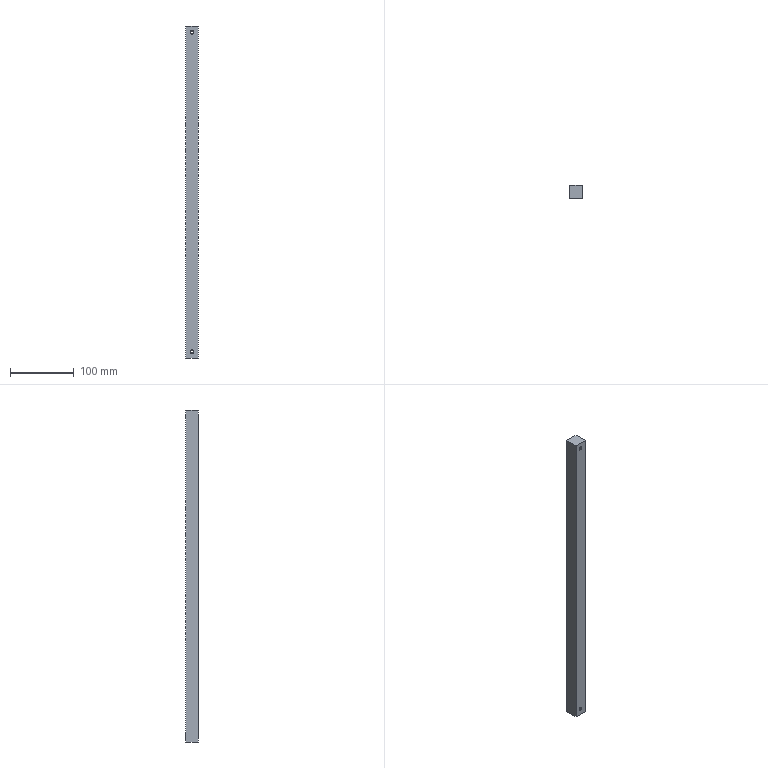Part | STEP file | Inner slide strip | 1 solid | 18 faces | box 20 x 20 x 520 mm | volume 207468 mm3 | cone 8 | plane 6 | cylinder 4 | commonest cylinder face diameters 4 x4
STEP:
#1=CARTESIAN_POINT('',(-3.247,0.9353,508.));
#2=VERTEX_POINT('',#1);
#3=CARTESIAN_POINT('',(-5.247,0.9353,510.));
#4=VERTEX_POINT('',#3);
#5=CARTESIAN_POINT('',(-3.247,0.9353,510.));
#6=DIRECTION('',(0.,1.,0.));
#7=DIRECTION('',(0.,0.,1.));
#8=AXIS2_PLACEMENT_3D('',#5,#6,#7);
#9=CIRCLE('',#8,2.);
#10=EDGE_CURVE('',#2,#4,#9,.T.);
#11=ORIENTED_EDGE('',*,*,#10,.F.);
#12=CARTESIAN_POINT('',(-3.247,1.935,507.));
#13=VERTEX_POINT('',#12);
#14=CARTESIAN_POINT('',(-3.247,1.935,507.));
#15=DIRECTION('',(0.,0.7071,-0.7071));
#16=VECTOR('',#15,1000.);
#17=LINE('',#14,#16);
#18=EDGE_CURVE('',#2,#13,#17,.T.);
#19=ORIENTED_EDGE('',*,*,#18,.T.);
#20=CARTESIAN_POINT('',(-3.247,1.935,513.));
#21=VERTEX_POINT('',#20);
#22=CARTESIAN_POINT('',(-3.247,1.935,510.));
#23=DIRECTION('',(0.,1.,0.));
#24=DIRECTION('',(0.,0.,1.));
#25=AXIS2_PLACEMENT_3D('',#22,#23,#24);
#26=CIRCLE('',#25,3.);
#27=EDGE_CURVE('',#13,#21,#26,.T.);
#28=ORIENTED_EDGE('',*,*,#27,.T.);
#29=CARTESIAN_POINT('',(-3.247,0.9353,512.));
#30=VERTEX_POINT('',#29);
#31=CARTESIAN_POINT('',(-3.247,1.935,513.));
#32=DIRECTION('',(0.,0.7071,0.7071));
#33=VECTOR('',#32,1000.);
#34=LINE('',#31,#33);
#35=EDGE_CURVE('',#30,#21,#34,.T.);
#36=ORIENTED_EDGE('',*,*,#35,.F.);
#37=CARTESIAN_POINT('',(-3.247,0.9353,510.));
#38=DIRECTION('',(0.,1.,0.));
#39=DIRECTION('',(0.,0.,1.));
#40=AXIS2_PLACEMENT_3D('',#37,#38,#39);
#41=CIRCLE('',#40,2.);
#42=EDGE_CURVE('',#4,#30,#41,.T.);
#43=ORIENTED_EDGE('',*,*,#42,.F.);
#44=EDGE_LOOP('',(#11,#19,#28,#36,#43));
#45=FACE_OUTER_BOUND('',#44,.T.);
#46=CARTESIAN_POINT('',(-3.247,1.935,510.));
#47=DIRECTION('',(0.,1.,0.));
#48=DIRECTION('',(0.,0.,1.));
#49=AXIS2_PLACEMENT_3D('',#46,#47,#48);
#50=CONICAL_SURFACE('',#49,3.,0.7854);
#51=ADVANCED_FACE('',(#45),#50,.F.);
#52=CARTESIAN_POINT('',(-3.247,0.9353,8.));
#53=VERTEX_POINT('',#52);
#54=CARTESIAN_POINT('',(-5.247,0.9353,10.));
#55=VERTEX_POINT('',#54);
#56=CARTESIAN_POINT('',(-3.247,0.9353,10.));
#57=DIRECTION('',(0.,1.,0.));
#58=DIRECTION('',(0.,0.,1.));
#59=AXIS2_PLACEMENT_3D('',#56,#57,#58);
#60=CIRCLE('',#59,2.);
#61=EDGE_CURVE('',#53,#55,#60,.T.);
#62=ORIENTED_EDGE('',*,*,#61,.F.);
#63=CARTESIAN_POINT('',(-3.247,1.935,7.));
#64=VERTEX_POINT('',#63);
#65=CARTESIAN_POINT('',(-3.247,1.935,7.));
#66=DIRECTION('',(0.,0.7071,-0.7071));
#67=VECTOR('',#66,1000.);
#68=LINE('',#65,#67);
#69=EDGE_CURVE('',#53,#64,#68,.T.);
#70=ORIENTED_EDGE('',*,*,#69,.T.);
#71=CARTESIAN_POINT('',(-3.247,1.935,13.));
#72=VERTEX_POINT('',#71);
#73=CARTESIAN_POINT('',(-3.247,1.935,10.));
#74=DIRECTION('',(0.,1.,0.));
#75=DIRECTION('',(0.,0.,1.));
#76=AXIS2_PLACEMENT_3D('',#73,#74,#75);
#77=CIRCLE('',#76,3.);
#78=EDGE_CURVE('',#64,#72,#77,.T.);
#79=ORIENTED_EDGE('',*,*,#78,.T.);
#80=CARTESIAN_POINT('',(-3.247,0.9353,12.));
#81=VERTEX_POINT('',#80);
#82=CARTESIAN_POINT('',(-3.247,1.935,13.));
#83=DIRECTION('',(0.,0.7071,0.7071));
#84=VECTOR('',#83,1000.);
#85=LINE('',#82,#84);
#86=EDGE_CURVE('',#81,#72,#85,.T.);
#87=ORIENTED_EDGE('',*,*,#86,.F.);
#88=CARTESIAN_POINT('',(-3.247,0.9353,10.));
#89=DIRECTION('',(0.,1.,0.));
#90=DIRECTION('',(0.,0.,1.));
#91=AXIS2_PLACEMENT_3D('',#88,#89,#90);
#92=CIRCLE('',#91,2.);
#93=EDGE_CURVE('',#55,#81,#92,.T.);
#94=ORIENTED_EDGE('',*,*,#93,.F.);
#95=EDGE_LOOP('',(#62,#70,#79,#87,#94));
#96=FACE_OUTER_BOUND('',#95,.T.);
#97=CARTESIAN_POINT('',(-3.247,1.935,10.));
#98=DIRECTION('',(0.,1.,0.));
#99=DIRECTION('',(0.,0.,1.));
#100=AXIS2_PLACEMENT_3D('',#97,#98,#99);
#101=CONICAL_SURFACE('',#100,3.,0.7854);
#102=ADVANCED_FACE('',(#96),#101,.F.);
#103=CARTESIAN_POINT('',(-3.247,-17.065,12.));
#104=VERTEX_POINT('',#103);
#105=CARTESIAN_POINT('',(-5.247,-17.065,10.));
#106=VERTEX_POINT('',#105);
#107=CARTESIAN_POINT('',(-3.247,-17.065,10.));
#108=DIRECTION('',(0.,-1.,0.));
#109=DIRECTION('',(0.,0.,-1.));
#110=AXIS2_PLACEMENT_3D('',#107,#108,#109);
#111=CIRCLE('',#110,2.);
#112=EDGE_CURVE('',#104,#106,#111,.T.);
#113=ORIENTED_EDGE('',*,*,#112,.F.);
#114=CARTESIAN_POINT('',(-3.247,-18.065,13.));
#115=VERTEX_POINT('',#114);
#116=CARTESIAN_POINT('',(-3.247,-18.065,13.));
#117=DIRECTION('',(0.,-0.7071,0.7071));
#118=VECTOR('',#117,1000.);
#119=LINE('',#116,#118);
#120=EDGE_CURVE('',#104,#115,#119,.T.);
#121=ORIENTED_EDGE('',*,*,#120,.T.);
#122=CARTESIAN_POINT('',(-3.247,-18.065,7.));
#123=VERTEX_POINT('',#122);
#124=CARTESIAN_POINT('',(-3.247,-18.065,10.));
#125=DIRECTION('',(0.,-1.,0.));
#126=DIRECTION('',(0.,0.,-1.));
#127=AXIS2_PLACEMENT_3D('',#124,#125,#126);
#128=CIRCLE('',#127,3.);
#129=EDGE_CURVE('',#115,#123,#128,.T.);
#130=ORIENTED_EDGE('',*,*,#129,.T.);
#131=CARTESIAN_POINT('',(-3.247,-17.065,8.));
#132=VERTEX_POINT('',#131);
#133=CARTESIAN_POINT('',(-3.247,-18.065,7.));
#134=DIRECTION('',(0.,-0.7071,-0.7071));
#135=VECTOR('',#134,1000.);
#136=LINE('',#133,#135);
#137=EDGE_CURVE('',#132,#123,#136,.T.);
#138=ORIENTED_EDGE('',*,*,#137,.F.);
#139=CARTESIAN_POINT('',(-3.247,-17.065,10.));
#140=DIRECTION('',(0.,-1.,0.));
#141=DIRECTION('',(0.,0.,-1.));
#142=AXIS2_PLACEMENT_3D('',#139,#140,#141);
#143=CIRCLE('',#142,2.);
#144=EDGE_CURVE('',#106,#132,#143,.T.);
#145=ORIENTED_EDGE('',*,*,#144,.F.);
#146=EDGE_LOOP('',(#113,#121,#130,#138,#145));
#147=FACE_OUTER_BOUND('',#146,.T.);
#148=CARTESIAN_POINT('',(-3.247,-18.065,10.));
#149=DIRECTION('',(0.,-1.,0.));
#150=DIRECTION('',(0.,0.,-1.));
#151=AXIS2_PLACEMENT_3D('',#148,#149,#150);
#152=CONICAL_SURFACE('',#151,3.,0.7854);
#153=ADVANCED_FACE('',(#147),#152,.F.);
#154=CARTESIAN_POINT('',(-3.247,-17.065,512.));
#155=VERTEX_POINT('',#154);
#156=CARTESIAN_POINT('',(-5.247,-17.065,510.));
#157=VERTEX_POINT('',#156);
#158=CARTESIAN_POINT('',(-3.247,-17.065,510.));
#159=DIRECTION('',(0.,-1.,0.));
#160=DIRECTION('',(0.,0.,-1.));
#161=AXIS2_PLACEMENT_3D('',#158,#159,#160);
#162=CIRCLE('',#161,2.);
#163=EDGE_CURVE('',#155,#157,#162,.T.);
#164=ORIENTED_EDGE('',*,*,#163,.F.);
#165=CARTESIAN_POINT('',(-3.247,-18.065,513.));
#166=VERTEX_POINT('',#165);
#167=CARTESIAN_POINT('',(-3.247,-18.065,513.));
#168=DIRECTION('',(0.,-0.7071,0.7071));
#169=VECTOR('',#168,1000.);
#170=LINE('',#167,#169);
#171=EDGE_CURVE('',#155,#166,#170,.T.);
#172=ORIENTED_EDGE('',*,*,#171,.T.);
#173=CARTESIAN_POINT('',(-3.247,-18.065,507.));
#174=VERTEX_POINT('',#173);
#175=CARTESIAN_POINT('',(-3.247,-18.065,510.));
#176=DIRECTION('',(0.,-1.,0.));
#177=DIRECTION('',(0.,0.,-1.));
#178=AXIS2_PLACEMENT_3D('',#175,#176,#177);
#179=CIRCLE('',#178,3.);
#180=EDGE_CURVE('',#166,#174,#179,.T.);
#181=ORIENTED_EDGE('',*,*,#180,.T.);
#182=CARTESIAN_POINT('',(-3.247,-17.065,508.));
#183=VERTEX_POINT('',#182);
#184=CARTESIAN_POINT('',(-3.247,-18.065,507.));
#185=DIRECTION('',(0.,-0.7071,-0.7071));
#186=VECTOR('',#185,1000.);
#187=LINE('',#184,#186);
#188=EDGE_CURVE('',#183,#174,#187,.T.);
#189=ORIENTED_EDGE('',*,*,#188,.F.);
#190=CARTESIAN_POINT('',(-3.247,-17.065,510.));
#191=DIRECTION('',(0.,-1.,0.));
#192=DIRECTION('',(0.,0.,-1.));
#193=AXIS2_PLACEMENT_3D('',#190,#191,#192);
#194=CIRCLE('',#193,2.);
#195=EDGE_CURVE('',#157,#183,#194,.T.);
#196=ORIENTED_EDGE('',*,*,#195,.F.);
#197=EDGE_LOOP('',(#164,#172,#181,#189,#196));
#198=FACE_OUTER_BOUND('',#197,.T.);
#199=CARTESIAN_POINT('',(-3.247,-18.065,510.));
#200=DIRECTION('',(0.,-1.,0.));
#201=DIRECTION('',(0.,0.,-1.));
#202=AXIS2_PLACEMENT_3D('',#199,#200,#201);
#203=CONICAL_SURFACE('',#202,3.,0.7854);
#204=ADVANCED_FACE('',(#198),#203,.F.);
#205=ORIENTED_EDGE('',*,*,#195,.T.);
#206=CARTESIAN_POINT('',(-1.247,-17.065,510.));
#207=VERTEX_POINT('',#206);
#208=CARTESIAN_POINT('',(-3.247,-17.065,510.));
#209=DIRECTION('',(0.,-1.,0.));
#210=DIRECTION('',(0.,0.,-1.));
#211=AXIS2_PLACEMENT_3D('',#208,#209,#210);
#212=CIRCLE('',#211,2.);
#213=EDGE_CURVE('',#183,#207,#212,.T.);
#214=ORIENTED_EDGE('',*,*,#213,.T.);
#215=CARTESIAN_POINT('',(-1.247,0.9353,510.));
#216=VERTEX_POINT('',#215);
#217=CARTESIAN_POINT('',(-1.247,-18.065,510.));
#218=DIRECTION('',(0.,1.,0.));
#219=VECTOR('',#218,1000.);
#220=LINE('',#217,#219);
#221=EDGE_CURVE('',#207,#216,#220,.T.);
#222=ORIENTED_EDGE('',*,*,#221,.T.);
#223=CARTESIAN_POINT('',(-3.247,0.9353,510.));
#224=DIRECTION('',(0.,1.,0.));
#225=DIRECTION('',(0.,0.,1.));
#226=AXIS2_PLACEMENT_3D('',#223,#224,#225);
#227=CIRCLE('',#226,2.);
#228=EDGE_CURVE('',#216,#2,#227,.T.);
#229=ORIENTED_EDGE('',*,*,#228,.T.);
#230=ORIENTED_EDGE('',*,*,#10,.T.);
#231=CARTESIAN_POINT('',(-5.247,-18.065,510.));
#232=DIRECTION('',(0.,1.,0.));
#233=VECTOR('',#232,1000.);
#234=LINE('',#231,#233);
#235=EDGE_CURVE('',#157,#4,#234,.T.);
#236=ORIENTED_EDGE('',*,*,#235,.F.);
#237=EDGE_LOOP('',(#205,#214,#222,#229,#230,#236));
#238=FACE_OUTER_BOUND('',#237,.T.);
#239=CARTESIAN_POINT('',(-3.247,-18.065,510.));
#240=DIRECTION('',(0.,1.,0.));
#241=DIRECTION('',(-1.,0.,0.));
#242=AXIS2_PLACEMENT_3D('',#239,#240,#241);
#243=CYLINDRICAL_SURFACE('',#242,2.);
#244=ADVANCED_FACE('',(#238),#243,.F.);
#245=ORIENTED_EDGE('',*,*,#144,.T.);
#246=CARTESIAN_POINT('',(-1.247,-17.065,10.));
#247=VERTEX_POINT('',#246);
#248=CARTESIAN_POINT('',(-3.247,-17.065,10.));
#249=DIRECTION('',(0.,-1.,0.));
#250=DIRECTION('',(0.,0.,-1.));
#251=AXIS2_PLACEMENT_3D('',#248,#249,#250);
#252=CIRCLE('',#251,2.);
#253=EDGE_CURVE('',#132,#247,#252,.T.);
#254=ORIENTED_EDGE('',*,*,#253,.T.);
#255=CARTESIAN_POINT('',(-1.247,0.9353,10.));
#256=VERTEX_POINT('',#255);
#257=CARTESIAN_POINT('',(-1.247,-18.065,10.));
#258=DIRECTION('',(0.,1.,0.));
#259=VECTOR('',#258,1000.);
#260=LINE('',#257,#259);
#261=EDGE_CURVE('',#247,#256,#260,.T.);
#262=ORIENTED_EDGE('',*,*,#261,.T.);
#263=CARTESIAN_POINT('',(-3.247,0.9353,10.));
#264=DIRECTION('',(0.,1.,0.));
#265=DIRECTION('',(0.,0.,1.));
#266=AXIS2_PLACEMENT_3D('',#263,#264,#265);
#267=CIRCLE('',#266,2.);
#268=EDGE_CURVE('',#256,#53,#267,.T.);
#269=ORIENTED_EDGE('',*,*,#268,.T.);
#270=ORIENTED_EDGE('',*,*,#61,.T.);
#271=CARTESIAN_POINT('',(-5.247,-18.065,10.));
#272=DIRECTION('',(0.,1.,0.));
#273=VECTOR('',#272,1000.);
#274=LINE('',#271,#273);
#275=EDGE_CURVE('',#106,#55,#274,.T.);
#276=ORIENTED_EDGE('',*,*,#275,.F.);
#277=EDGE_LOOP('',(#245,#254,#262,#269,#270,#276));
#278=FACE_OUTER_BOUND('',#277,.T.);
#279=CARTESIAN_POINT('',(-3.247,-18.065,10.));
#280=DIRECTION('',(0.,1.,0.));
#281=DIRECTION('',(-1.,0.,0.));
#282=AXIS2_PLACEMENT_3D('',#279,#280,#281);
#283=CYLINDRICAL_SURFACE('',#282,2.);
#284=ADVANCED_FACE('',(#278),#283,.F.);
#285=CARTESIAN_POINT('',(6.753,1.935,520.));
#286=VERTEX_POINT('',#285);
#287=CARTESIAN_POINT('',(6.753,1.935,0.));
#288=VERTEX_POINT('',#287);
#289=CARTESIAN_POINT('',(6.753,1.935,520.));
#290=DIRECTION('',(0.,0.,-1.));
#291=VECTOR('',#290,1000.);
#292=LINE('',#289,#291);
#293=EDGE_CURVE('',#286,#288,#292,.T.);
#294=ORIENTED_EDGE('',*,*,#293,.F.);
#295=CARTESIAN_POINT('',(6.753,-18.065,520.));
#296=VERTEX_POINT('',#295);
#297=CARTESIAN_POINT('',(6.753,1.935,520.));
#298=DIRECTION('',(0.,1.,0.));
#299=VECTOR('',#298,1000.);
#300=LINE('',#297,#299);
#301=EDGE_CURVE('',#296,#286,#300,.T.);
#302=ORIENTED_EDGE('',*,*,#301,.F.);
#303=CARTESIAN_POINT('',(6.753,-18.065,0.));
#304=VERTEX_POINT('',#303);
#305=CARTESIAN_POINT('',(6.753,-18.065,520.));
#306=DIRECTION('',(0.,0.,1.));
#307=VECTOR('',#306,1000.);
#308=LINE('',#305,#307);
#309=EDGE_CURVE('',#304,#296,#308,.T.);
#310=ORIENTED_EDGE('',*,*,#309,.F.);
#311=CARTESIAN_POINT('',(6.753,1.935,0.));
#312=DIRECTION('',(0.,-1.,0.));
#313=VECTOR('',#312,1000.);
#314=LINE('',#311,#313);
#315=EDGE_CURVE('',#288,#304,#314,.T.);
#316=ORIENTED_EDGE('',*,*,#315,.F.);
#317=EDGE_LOOP('',(#294,#302,#310,#316));
#318=FACE_OUTER_BOUND('',#317,.T.);
#319=CARTESIAN_POINT('',(6.753,1.935,520.));
#320=DIRECTION('',(-1.,0.,0.));
#321=DIRECTION('',(0.,0.,1.));
#322=AXIS2_PLACEMENT_3D('',#319,#320,#321);
#323=PLANE('',#322);
#324=ADVANCED_FACE('',(#318),#323,.F.);
#325=CARTESIAN_POINT('',(-13.247,1.935,0.));
#326=VERTEX_POINT('',#325);
#327=CARTESIAN_POINT('',(-13.247,1.935,0.));
#328=DIRECTION('',(-1.,0.,0.));
#329=VECTOR('',#328,1000.);
#330=LINE('',#327,#329);
#331=EDGE_CURVE('',#288,#326,#330,.T.);
#332=ORIENTED_EDGE('',*,*,#331,.F.);
#333=ORIENTED_EDGE('',*,*,#315,.T.);
#334=CARTESIAN_POINT('',(-13.247,-18.065,0.));
#335=VERTEX_POINT('',#334);
#336=CARTESIAN_POINT('',(-13.247,-18.065,0.));
#337=DIRECTION('',(1.,0.,0.));
#338=VECTOR('',#337,1000.);
#339=LINE('',#336,#338);
#340=EDGE_CURVE('',#335,#304,#339,.T.);
#341=ORIENTED_EDGE('',*,*,#340,.F.);
#342=CARTESIAN_POINT('',(-13.247,-18.065,0.));
#343=DIRECTION('',(0.,-1.,0.));
#344=VECTOR('',#343,1000.);
#345=LINE('',#342,#344);
#346=EDGE_CURVE('',#326,#335,#345,.T.);
#347=ORIENTED_EDGE('',*,*,#346,.F.);
#348=EDGE_LOOP('',(#332,#333,#341,#347));
#349=FACE_OUTER_BOUND('',#348,.T.);
#350=CARTESIAN_POINT('',(-13.247,-18.065,0.));
#351=DIRECTION('',(0.,0.,1.));
#352=DIRECTION('',(1.,0.,0.));
#353=AXIS2_PLACEMENT_3D('',#350,#351,#352);
#354=PLANE('',#353);
#355=ADVANCED_FACE('',(#349),#354,.F.);
#356=CARTESIAN_POINT('',(-13.247,1.935,520.));
#357=VERTEX_POINT('',#356);
#358=CARTESIAN_POINT('',(-13.247,1.935,520.));
#359=DIRECTION('',(0.,0.,-1.));
#360=VECTOR('',#359,1000.);
#361=LINE('',#358,#360);
#362=EDGE_CURVE('',#357,#326,#361,.T.);
#363=ORIENTED_EDGE('',*,*,#362,.F.);
#364=CARTESIAN_POINT('',(-13.247,1.935,520.));
#365=DIRECTION('',(-1.,0.,0.));
#366=VECTOR('',#365,1000.);
#367=LINE('',#364,#366);
#368=EDGE_CURVE('',#286,#357,#367,.T.);
#369=ORIENTED_EDGE('',*,*,#368,.F.);
#370=ORIENTED_EDGE('',*,*,#293,.T.);
#371=ORIENTED_EDGE('',*,*,#331,.T.);
#372=EDGE_LOOP('',(#363,#369,#370,#371));
#373=FACE_OUTER_BOUND('',#372,.T.);
#374=CARTESIAN_POINT('',(-3.247,1.935,510.));
#375=DIRECTION('',(0.,1.,0.));
#376=DIRECTION('',(0.,0.,1.));
#377=AXIS2_PLACEMENT_3D('',#374,#375,#376);
#378=CIRCLE('',#377,3.);
#379=EDGE_CURVE('',#21,#13,#378,.T.);
#380=ORIENTED_EDGE('',*,*,#379,.F.);
#381=ORIENTED_EDGE('',*,*,#27,.F.);
#382=EDGE_LOOP('',(#380,#381));
#383=FACE_BOUND('',#382,.T.);
#384=CARTESIAN_POINT('',(-3.247,1.935,10.));
#385=DIRECTION('',(0.,1.,0.));
#386=DIRECTION('',(0.,0.,1.));
#387=AXIS2_PLACEMENT_3D('',#384,#385,#386);
#388=CIRCLE('',#387,3.);
#389=EDGE_CURVE('',#72,#64,#388,.T.);
#390=ORIENTED_EDGE('',*,*,#389,.F.);
#391=ORIENTED_EDGE('',*,*,#78,.F.);
#392=EDGE_LOOP('',(#390,#391));
#393=FACE_BOUND('',#392,.T.);
#394=CARTESIAN_POINT('',(-13.247,1.935,520.));
#395=DIRECTION('',(0.,-1.,0.));
#396=DIRECTION('',(1.,0.,0.));
#397=AXIS2_PLACEMENT_3D('',#394,#395,#396);
#398=PLANE('',#397);
#399=ADVANCED_FACE('',(#373,#383,#393),#398,.F.);
#400=ORIENTED_EDGE('',*,*,#301,.T.);
#401=ORIENTED_EDGE('',*,*,#368,.T.);
#402=CARTESIAN_POINT('',(-13.247,-18.065,520.));
#403=VERTEX_POINT('',#402);
#404=CARTESIAN_POINT('',(-13.247,-18.065,520.));
#405=DIRECTION('',(0.,-1.,0.));
#406=VECTOR('',#405,1000.);
#407=LINE('',#404,#406);
#408=EDGE_CURVE('',#357,#403,#407,.T.);
#409=ORIENTED_EDGE('',*,*,#408,.T.);
#410=CARTESIAN_POINT('',(-13.247,-18.065,520.));
#411=DIRECTION('',(1.,0.,0.));
#412=VECTOR('',#411,1000.);
#413=LINE('',#410,#412);
#414=EDGE_CURVE('',#403,#296,#413,.T.);
#415=ORIENTED_EDGE('',*,*,#414,.T.);
#416=EDGE_LOOP('',(#400,#401,#409,#415));
#417=FACE_OUTER_BOUND('',#416,.T.);
#418=CARTESIAN_POINT('',(-13.247,-18.065,520.));
#419=DIRECTION('',(0.,0.,1.));
#420=DIRECTION('',(1.,0.,0.));
#421=AXIS2_PLACEMENT_3D('',#418,#419,#420);
#422=PLANE('',#421);
#423=ADVANCED_FACE('',(#417),#422,.T.);
#424=ORIENTED_EDGE('',*,*,#309,.T.);
#425=ORIENTED_EDGE('',*,*,#414,.F.);
#426=CARTESIAN_POINT('',(-13.247,-18.065,520.));
#427=DIRECTION('',(0.,0.,1.));
#428=VECTOR('',#427,1000.);
#429=LINE('',#426,#428);
#430=EDGE_CURVE('',#335,#403,#429,.T.);
#431=ORIENTED_EDGE('',*,*,#430,.F.);
#432=ORIENTED_EDGE('',*,*,#340,.T.);
#433=EDGE_LOOP('',(#424,#425,#431,#432));
#434=FACE_OUTER_BOUND('',#433,.T.);
#435=CARTESIAN_POINT('',(-3.247,-18.065,10.));
#436=DIRECTION('',(0.,-1.,0.));
#437=DIRECTION('',(0.,0.,-1.));
#438=AXIS2_PLACEMENT_3D('',#435,#436,#437);
#439=CIRCLE('',#438,3.);
#440=EDGE_CURVE('',#123,#115,#439,.T.);
#441=ORIENTED_EDGE('',*,*,#440,.F.);
#442=ORIENTED_EDGE('',*,*,#129,.F.);
#443=EDGE_LOOP('',(#441,#442));
#444=FACE_BOUND('',#443,.T.);
#445=CARTESIAN_POINT('',(-3.247,-18.065,510.));
#446=DIRECTION('',(0.,-1.,0.));
#447=DIRECTION('',(0.,0.,-1.));
#448=AXIS2_PLACEMENT_3D('',#445,#446,#447);
#449=CIRCLE('',#448,3.);
#450=EDGE_CURVE('',#174,#166,#449,.T.);
#451=ORIENTED_EDGE('',*,*,#450,.F.);
#452=ORIENTED_EDGE('',*,*,#180,.F.);
#453=EDGE_LOOP('',(#451,#452));
#454=FACE_BOUND('',#453,.T.);
#455=CARTESIAN_POINT('',(-13.247,-18.065,520.));
#456=DIRECTION('',(0.,1.,0.));
#457=DIRECTION('',(0.,0.,1.));
#458=AXIS2_PLACEMENT_3D('',#455,#456,#457);
#459=PLANE('',#458);
#460=ADVANCED_FACE('',(#434,#444,#454),#459,.F.);
#461=ORIENTED_EDGE('',*,*,#430,.T.);
#462=ORIENTED_EDGE('',*,*,#408,.F.);
#463=ORIENTED_EDGE('',*,*,#362,.T.);
#464=ORIENTED_EDGE('',*,*,#346,.T.);
#465=EDGE_LOOP('',(#461,#462,#463,#464));
#466=FACE_OUTER_BOUND('',#465,.T.);
#467=CARTESIAN_POINT('',(-13.247,1.935,520.));
#468=DIRECTION('',(1.,0.,0.));
#469=DIRECTION('',(0.,0.,-1.));
#470=AXIS2_PLACEMENT_3D('',#467,#468,#469);
#471=PLANE('',#470);
#472=ADVANCED_FACE('',(#466),#471,.F.);
#473=ORIENTED_EDGE('',*,*,#18,.F.);
#474=ORIENTED_EDGE('',*,*,#228,.F.);
#475=CARTESIAN_POINT('',(-3.247,0.9353,510.));
#476=DIRECTION('',(0.,1.,0.));
#477=DIRECTION('',(0.,0.,1.));
#478=AXIS2_PLACEMENT_3D('',#475,#476,#477);
#479=CIRCLE('',#478,2.);
#480=EDGE_CURVE('',#30,#216,#479,.T.);
#481=ORIENTED_EDGE('',*,*,#480,.F.);
#482=ORIENTED_EDGE('',*,*,#35,.T.);
#483=ORIENTED_EDGE('',*,*,#379,.T.);
#484=EDGE_LOOP('',(#473,#474,#481,#482,#483));
#485=FACE_OUTER_BOUND('',#484,.T.);
#486=CARTESIAN_POINT('',(-3.247,1.935,510.));
#487=DIRECTION('',(0.,1.,0.));
#488=DIRECTION('',(0.,0.,1.));
#489=AXIS2_PLACEMENT_3D('',#486,#487,#488);
#490=CONICAL_SURFACE('',#489,3.,0.7854);
#491=ADVANCED_FACE('',(#485),#490,.F.);
#492=ORIENTED_EDGE('',*,*,#69,.F.);
#493=ORIENTED_EDGE('',*,*,#268,.F.);
#494=CARTESIAN_POINT('',(-3.247,0.9353,10.));
#495=DIRECTION('',(0.,1.,0.));
#496=DIRECTION('',(0.,0.,1.));
#497=AXIS2_PLACEMENT_3D('',#494,#495,#496);
#498=CIRCLE('',#497,2.);
#499=EDGE_CURVE('',#81,#256,#498,.T.);
#500=ORIENTED_EDGE('',*,*,#499,.F.);
#501=ORIENTED_EDGE('',*,*,#86,.T.);
#502=ORIENTED_EDGE('',*,*,#389,.T.);
#503=EDGE_LOOP('',(#492,#493,#500,#501,#502));
#504=FACE_OUTER_BOUND('',#503,.T.);
#505=CARTESIAN_POINT('',(-3.247,1.935,10.));
#506=DIRECTION('',(0.,1.,0.));
#507=DIRECTION('',(0.,0.,1.));
#508=AXIS2_PLACEMENT_3D('',#505,#506,#507);
#509=CONICAL_SURFACE('',#508,3.,0.7854);
#510=ADVANCED_FACE('',(#504),#509,.F.);
#511=ORIENTED_EDGE('',*,*,#120,.F.);
#512=CARTESIAN_POINT('',(-3.247,-17.065,10.));
#513=DIRECTION('',(0.,-1.,0.));
#514=DIRECTION('',(0.,0.,-1.));
#515=AXIS2_PLACEMENT_3D('',#512,#513,#514);
#516=CIRCLE('',#515,2.);
#517=EDGE_CURVE('',#247,#104,#516,.T.);
#518=ORIENTED_EDGE('',*,*,#517,.F.);
#519=ORIENTED_EDGE('',*,*,#253,.F.);
#520=ORIENTED_EDGE('',*,*,#137,.T.);
#521=ORIENTED_EDGE('',*,*,#440,.T.);
#522=EDGE_LOOP('',(#511,#518,#519,#520,#521));
#523=FACE_OUTER_BOUND('',#522,.T.);
#524=CARTESIAN_POINT('',(-3.247,-18.065,10.));
#525=DIRECTION('',(0.,-1.,0.));
#526=DIRECTION('',(0.,0.,-1.));
#527=AXIS2_PLACEMENT_3D('',#524,#525,#526);
#528=CONICAL_SURFACE('',#527,3.,0.7854);
#529=ADVANCED_FACE('',(#523),#528,.F.);
#530=ORIENTED_EDGE('',*,*,#171,.F.);
#531=CARTESIAN_POINT('',(-3.247,-17.065,510.));
#532=DIRECTION('',(0.,-1.,0.));
#533=DIRECTION('',(0.,0.,-1.));
#534=AXIS2_PLACEMENT_3D('',#531,#532,#533);
#535=CIRCLE('',#534,2.);
#536=EDGE_CURVE('',#207,#155,#535,.T.);
#537=ORIENTED_EDGE('',*,*,#536,.F.);
#538=ORIENTED_EDGE('',*,*,#213,.F.);
#539=ORIENTED_EDGE('',*,*,#188,.T.);
#540=ORIENTED_EDGE('',*,*,#450,.T.);
#541=EDGE_LOOP('',(#530,#537,#538,#539,#540));
#542=FACE_OUTER_BOUND('',#541,.T.);
#543=CARTESIAN_POINT('',(-3.247,-18.065,510.));
#544=DIRECTION('',(0.,-1.,0.));
#545=DIRECTION('',(0.,0.,-1.));
#546=AXIS2_PLACEMENT_3D('',#543,#544,#545);
#547=CONICAL_SURFACE('',#546,3.,0.7854);
#548=ADVANCED_FACE('',(#542),#547,.F.);
#549=ORIENTED_EDGE('',*,*,#221,.F.);
#550=ORIENTED_EDGE('',*,*,#536,.T.);
#551=ORIENTED_EDGE('',*,*,#163,.T.);
#552=ORIENTED_EDGE('',*,*,#235,.T.);
#553=ORIENTED_EDGE('',*,*,#42,.T.);
#554=ORIENTED_EDGE('',*,*,#480,.T.);
#555=EDGE_LOOP('',(#549,#550,#551,#552,#553,#554));
#556=FACE_OUTER_BOUND('',#555,.T.);
#557=CARTESIAN_POINT('',(-3.247,-18.065,510.));
#558=DIRECTION('',(0.,1.,0.));
#559=DIRECTION('',(-1.,0.,0.));
#560=AXIS2_PLACEMENT_3D('',#557,#558,#559);
#561=CYLINDRICAL_SURFACE('',#560,2.);
#562=ADVANCED_FACE('',(#556),#561,.F.);
#563=ORIENTED_EDGE('',*,*,#261,.F.);
#564=ORIENTED_EDGE('',*,*,#517,.T.);
#565=ORIENTED_EDGE('',*,*,#112,.T.);
#566=ORIENTED_EDGE('',*,*,#275,.T.);
#567=ORIENTED_EDGE('',*,*,#93,.T.);
#568=ORIENTED_EDGE('',*,*,#499,.T.);
#569=EDGE_LOOP('',(#563,#564,#565,#566,#567,#568));
#570=FACE_OUTER_BOUND('',#569,.T.);
#571=CARTESIAN_POINT('',(-3.247,-18.065,10.));
#572=DIRECTION('',(0.,1.,0.));
#573=DIRECTION('',(-1.,0.,0.));
#574=AXIS2_PLACEMENT_3D('',#571,#572,#573);
#575=CYLINDRICAL_SURFACE('',#574,2.);
#576=ADVANCED_FACE('',(#570),#575,.F.);
#577=CLOSED_SHELL('',(#51,#102,#153,#204,#244,#284,#324,#355,#399,#423,#460,#472,#491,#510,#529,#548,#562,#576));
#578=MANIFOLD_SOLID_BREP('',#577);
#579=CARTESIAN_POINT('',(0.,0.,0.));
#580=DIRECTION('',(0.,0.,1.));
#581=DIRECTION('',(1.,0.,0.));
#582=AXIS2_PLACEMENT_3D('',#579,#580,#581);
#583=(LENGTH_UNIT()NAMED_UNIT(*)SI_UNIT(.MILLI.,.METRE.));
#584=UNCERTAINTY_MEASURE_WITH_UNIT(LENGTH_MEASURE(0.00001),#583,'','');
#585=(NAMED_UNIT(*)PLANE_ANGLE_UNIT()SI_UNIT($,.RADIAN.));
#586=(NAMED_UNIT(*)SI_UNIT($,.STERADIAN.)SOLID_ANGLE_UNIT());
#587=(GEOMETRIC_REPRESENTATION_CONTEXT(3)GLOBAL_UNCERTAINTY_ASSIGNED_CONTEXT((#584))GLOBAL_UNIT_ASSIGNED_CONTEXT((#583,#585,#586))REPRESENTATION_CONTEXT('',''));
#588=ADVANCED_BREP_SHAPE_REPRESENTATION('',(#578,#582),#587);